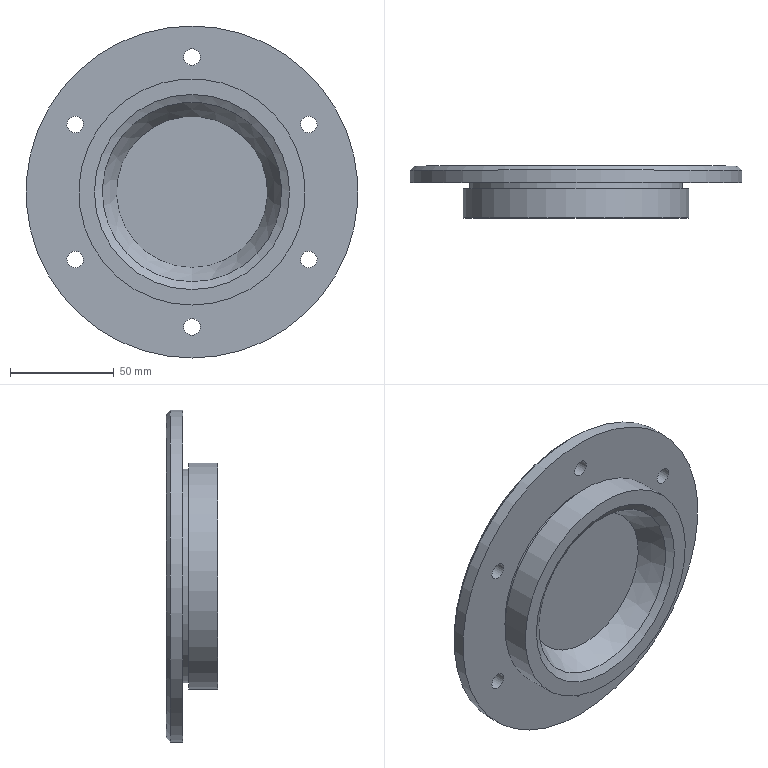Part | NX | features DATUM_CSYS 3, EXTRUDE 3, SKETCH 2, BREP 1 | 1 solid | 19 faces | box 160 x 25 x 160 mm | volume 214093 mm3 | cylinder 9 | plane 6 | cone 4 | commonest cylinder face diameters 8 x6 103 x1 109 x1 160 x1
STEP:
#1=CARTESIAN_POINT('',(0.5,681.,-36.417));
#2=VERTEX_POINT('',#1);
#3=CARTESIAN_POINT('',(0.5,681.,0.));
#4=DIRECTION('',(0.,-1.,0.));
#5=DIRECTION('',(0.,0.,-1.));
#6=AXIS2_PLACEMENT_3D('',#3,#4,#5);
#7=CIRCLE('',#6,36.417);
#8=EDGE_CURVE('',#2,#2,#7,.T.);
#9=ORIENTED_EDGE('',*,*,#8,.F.);
#10=EDGE_LOOP('',(#9));
#11=FACE_BOUND('',#10,.T.);
#12=CARTESIAN_POINT('',(0.5,669.165,-43.25));
#13=VERTEX_POINT('',#12);
#14=CARTESIAN_POINT('',(0.5,669.165,0.));
#15=DIRECTION('',(0.,-1.,0.));
#16=DIRECTION('',(0.,0.,-1.));
#17=AXIS2_PLACEMENT_3D('',#14,#15,#16);
#18=CIRCLE('',#17,43.25);
#19=EDGE_CURVE('',#13,#13,#18,.T.);
#20=ORIENTED_EDGE('',*,*,#19,.T.);
#21=EDGE_LOOP('',(#20));
#22=FACE_BOUND('',#21,.T.);
#23=CARTESIAN_POINT('',(0.5,669.165,0.));
#24=DIRECTION('',(0.,-1.,0.));
#25=DIRECTION('',(0.,0.,-1.));
#26=AXIS2_PLACEMENT_3D('',#23,#24,#25);
#27=CONICAL_SURFACE('',#26,43.25,0.5236);
#28=ADVANCED_FACE('',(#11,#22),#27,.F.);
#29=ORIENTED_EDGE('',*,*,#8,.T.);
#30=EDGE_LOOP('',(#29));
#31=FACE_BOUND('',#30,.T.);
#32=CARTESIAN_POINT('',(36.917,681.,0.));
#33=DIRECTION('',(0.,1.,0.));
#34=DIRECTION('',(0.,0.,1.));
#35=AXIS2_PLACEMENT_3D('',#32,#33,#34);
#36=PLANE('',#35);
#37=ADVANCED_FACE('',(#31),#36,.F.);
#38=CARTESIAN_POINT('',(0.5,689.,-51.));
#39=VERTEX_POINT('',#38);
#40=CARTESIAN_POINT('',(0.5,689.,0.));
#41=DIRECTION('',(0.,-1.,0.));
#42=DIRECTION('',(0.,0.,-1.));
#43=AXIS2_PLACEMENT_3D('',#40,#41,#42);
#44=CIRCLE('',#43,51.);
#45=EDGE_CURVE('',#39,#39,#44,.T.);
#46=ORIENTED_EDGE('',*,*,#45,.F.);
#47=EDGE_LOOP('',(#46));
#48=FACE_BOUND('',#47,.T.);
#49=CARTESIAN_POINT('',(0.5,689.,0.));
#50=DIRECTION('',(0.,-1.,0.));
#51=DIRECTION('',(0.,0.,-1.));
#52=AXIS2_PLACEMENT_3D('',#49,#50,#51);
#53=PLANE('',#52);
#54=ADVANCED_FACE('',(#48),#53,.F.);
#55=CARTESIAN_POINT('',(0.5,692.,-54.));
#56=VERTEX_POINT('',#55);
#57=CARTESIAN_POINT('',(0.5,692.,0.));
#58=DIRECTION('',(0.,-1.,0.));
#59=DIRECTION('',(0.,0.,-1.));
#60=AXIS2_PLACEMENT_3D('',#57,#58,#59);
#61=CIRCLE('',#60,54.);
#62=EDGE_CURVE('',#56,#56,#61,.T.);
#63=ORIENTED_EDGE('',*,*,#62,.F.);
#64=EDGE_LOOP('',(#63));
#65=FACE_BOUND('',#64,.T.);
#66=ORIENTED_EDGE('',*,*,#45,.T.);
#67=EDGE_LOOP('',(#66));
#68=FACE_BOUND('',#67,.T.);
#69=CARTESIAN_POINT('',(0.5,689.,0.));
#70=DIRECTION('',(0.,1.,0.));
#71=DIRECTION('',(0.,0.,1.));
#72=AXIS2_PLACEMENT_3D('',#69,#70,#71);
#73=CONICAL_SURFACE('',#72,51.,0.7854);
#74=ADVANCED_FACE('',(#65,#68),#73,.F.);
#75=CARTESIAN_POINT('',(-57.792,692.,29.036));
#76=VERTEX_POINT('',#75);
#77=CARTESIAN_POINT('',(-55.792,692.,32.5));
#78=DIRECTION('',(0.,1.,0.));
#79=DIRECTION('',(-0.5,0.,-0.866));
#80=AXIS2_PLACEMENT_3D('',#77,#78,#79);
#81=CIRCLE('',#80,4.);
#82=EDGE_CURVE('',#76,#76,#81,.T.);
#83=ORIENTED_EDGE('',*,*,#82,.F.);
#84=EDGE_LOOP('',(#83));
#85=FACE_BOUND('',#84,.T.);
#86=CARTESIAN_POINT('',(4.5,692.,-65.));
#87=VERTEX_POINT('',#86);
#88=CARTESIAN_POINT('',(0.5,692.,-65.));
#89=DIRECTION('',(0.,1.,0.));
#90=DIRECTION('',(1.,0.,0.));
#91=AXIS2_PLACEMENT_3D('',#88,#89,#90);
#92=CIRCLE('',#91,4.);
#93=EDGE_CURVE('',#87,#87,#92,.T.);
#94=ORIENTED_EDGE('',*,*,#93,.F.);
#95=EDGE_LOOP('',(#94));
#96=FACE_BOUND('',#95,.T.);
#97=CARTESIAN_POINT('',(-3.5,692.,65.));
#98=VERTEX_POINT('',#97);
#99=CARTESIAN_POINT('',(0.5,692.,65.));
#100=DIRECTION('',(0.,1.,0.));
#101=DIRECTION('',(-1.,0.,0.));
#102=AXIS2_PLACEMENT_3D('',#99,#100,#101);
#103=CIRCLE('',#102,4.);
#104=EDGE_CURVE('',#98,#98,#103,.T.);
#105=ORIENTED_EDGE('',*,*,#104,.F.);
#106=EDGE_LOOP('',(#105));
#107=FACE_BOUND('',#106,.T.);
#108=CARTESIAN_POINT('',(58.792,692.,-29.036));
#109=VERTEX_POINT('',#108);
#110=CARTESIAN_POINT('',(56.792,692.,-32.5));
#111=DIRECTION('',(0.,1.,0.));
#112=DIRECTION('',(0.5,0.,0.866));
#113=AXIS2_PLACEMENT_3D('',#110,#111,#112);
#114=CIRCLE('',#113,4.);
#115=EDGE_CURVE('',#109,#109,#114,.T.);
#116=ORIENTED_EDGE('',*,*,#115,.F.);
#117=EDGE_LOOP('',(#116));
#118=FACE_BOUND('',#117,.T.);
#119=CARTESIAN_POINT('',(-53.792,692.,-35.964));
#120=VERTEX_POINT('',#119);
#121=CARTESIAN_POINT('',(-55.792,692.,-32.5));
#122=DIRECTION('',(0.,1.,0.));
#123=DIRECTION('',(0.5,0.,-0.866));
#124=AXIS2_PLACEMENT_3D('',#121,#122,#123);
#125=CIRCLE('',#124,4.);
#126=EDGE_CURVE('',#120,#120,#125,.T.);
#127=ORIENTED_EDGE('',*,*,#126,.F.);
#128=EDGE_LOOP('',(#127));
#129=FACE_BOUND('',#128,.T.);
#130=CARTESIAN_POINT('',(54.792,692.,35.964));
#131=VERTEX_POINT('',#130);
#132=CARTESIAN_POINT('',(56.792,692.,32.5));
#133=DIRECTION('',(0.,1.,0.));
#134=DIRECTION('',(-0.5,0.,0.866));
#135=AXIS2_PLACEMENT_3D('',#132,#133,#134);
#136=CIRCLE('',#135,4.);
#137=EDGE_CURVE('',#131,#131,#136,.T.);
#138=ORIENTED_EDGE('',*,*,#137,.F.);
#139=EDGE_LOOP('',(#138));
#140=FACE_BOUND('',#139,.T.);
#141=CARTESIAN_POINT('',(0.5,692.,-78.));
#142=VERTEX_POINT('',#141);
#143=CARTESIAN_POINT('',(0.5,692.,0.));
#144=DIRECTION('',(0.,-1.,0.));
#145=DIRECTION('',(0.,0.,-1.));
#146=AXIS2_PLACEMENT_3D('',#143,#144,#145);
#147=CIRCLE('',#146,78.);
#148=EDGE_CURVE('',#142,#142,#147,.T.);
#149=ORIENTED_EDGE('',*,*,#148,.F.);
#150=EDGE_LOOP('',(#149));
#151=FACE_BOUND('',#150,.T.);
#152=ORIENTED_EDGE('',*,*,#62,.T.);
#153=EDGE_LOOP('',(#152));
#154=FACE_BOUND('',#153,.T.);
#155=CARTESIAN_POINT('',(54.5,692.,0.));
#156=DIRECTION('',(0.,-1.,0.));
#157=DIRECTION('',(0.,0.,-1.));
#158=AXIS2_PLACEMENT_3D('',#155,#156,#157);
#159=PLANE('',#158);
#160=ADVANCED_FACE('',(#85,#96,#107,#118,#129,#140,#151,#154),#159,.F.);
#161=CARTESIAN_POINT('',(0.5,690.,-80.));
#162=VERTEX_POINT('',#161);
#163=CARTESIAN_POINT('',(0.5,690.,0.));
#164=DIRECTION('',(0.,-1.,0.));
#165=DIRECTION('',(0.,0.,-1.));
#166=AXIS2_PLACEMENT_3D('',#163,#164,#165);
#167=CIRCLE('',#166,80.);
#168=EDGE_CURVE('',#162,#162,#167,.T.);
#169=ORIENTED_EDGE('',*,*,#168,.F.);
#170=EDGE_LOOP('',(#169));
#171=FACE_BOUND('',#170,.T.);
#172=ORIENTED_EDGE('',*,*,#148,.T.);
#173=EDGE_LOOP('',(#172));
#174=FACE_BOUND('',#173,.T.);
#175=CARTESIAN_POINT('',(0.5,692.,0.));
#176=DIRECTION('',(0.,-1.,0.));
#177=DIRECTION('',(0.,0.,-1.));
#178=AXIS2_PLACEMENT_3D('',#175,#176,#177);
#179=CONICAL_SURFACE('',#178,78.,0.7854);
#180=ADVANCED_FACE('',(#171,#174),#179,.T.);
#181=CARTESIAN_POINT('',(0.5,684.,-80.));
#182=VERTEX_POINT('',#181);
#183=CARTESIAN_POINT('',(0.5,684.,0.));
#184=DIRECTION('',(0.,-1.,0.));
#185=DIRECTION('',(0.,0.,-1.));
#186=AXIS2_PLACEMENT_3D('',#183,#184,#185);
#187=CIRCLE('',#186,80.);
#188=EDGE_CURVE('',#182,#182,#187,.T.);
#189=ORIENTED_EDGE('',*,*,#188,.F.);
#190=EDGE_LOOP('',(#189));
#191=FACE_BOUND('',#190,.T.);
#192=ORIENTED_EDGE('',*,*,#168,.T.);
#193=EDGE_LOOP('',(#192));
#194=FACE_BOUND('',#193,.T.);
#195=CARTESIAN_POINT('',(0.5,681.,0.));
#196=DIRECTION('',(0.,-1.,0.));
#197=DIRECTION('',(0.,0.,-1.));
#198=AXIS2_PLACEMENT_3D('',#195,#196,#197);
#199=CYLINDRICAL_SURFACE('',#198,80.);
#200=ADVANCED_FACE('',(#191,#194),#199,.T.);
#201=CARTESIAN_POINT('',(-57.792,684.,29.036));
#202=VERTEX_POINT('',#201);
#203=CARTESIAN_POINT('',(-55.792,684.,32.5));
#204=DIRECTION('',(0.,1.,0.));
#205=DIRECTION('',(-0.5,0.,-0.866));
#206=AXIS2_PLACEMENT_3D('',#203,#204,#205);
#207=CIRCLE('',#206,4.);
#208=EDGE_CURVE('',#202,#202,#207,.T.);
#209=ORIENTED_EDGE('',*,*,#208,.T.);
#210=EDGE_LOOP('',(#209));
#211=FACE_BOUND('',#210,.T.);
#212=CARTESIAN_POINT('',(4.5,684.,-65.));
#213=VERTEX_POINT('',#212);
#214=CARTESIAN_POINT('',(0.5,684.,-65.));
#215=DIRECTION('',(0.,1.,0.));
#216=DIRECTION('',(1.,0.,0.));
#217=AXIS2_PLACEMENT_3D('',#214,#215,#216);
#218=CIRCLE('',#217,4.);
#219=EDGE_CURVE('',#213,#213,#218,.T.);
#220=ORIENTED_EDGE('',*,*,#219,.T.);
#221=EDGE_LOOP('',(#220));
#222=FACE_BOUND('',#221,.T.);
#223=CARTESIAN_POINT('',(-3.5,684.,65.));
#224=VERTEX_POINT('',#223);
#225=CARTESIAN_POINT('',(0.5,684.,65.));
#226=DIRECTION('',(0.,1.,0.));
#227=DIRECTION('',(-1.,0.,0.));
#228=AXIS2_PLACEMENT_3D('',#225,#226,#227);
#229=CIRCLE('',#228,4.);
#230=EDGE_CURVE('',#224,#224,#229,.T.);
#231=ORIENTED_EDGE('',*,*,#230,.T.);
#232=EDGE_LOOP('',(#231));
#233=FACE_BOUND('',#232,.T.);
#234=CARTESIAN_POINT('',(58.792,684.,-29.036));
#235=VERTEX_POINT('',#234);
#236=CARTESIAN_POINT('',(56.792,684.,-32.5));
#237=DIRECTION('',(0.,1.,0.));
#238=DIRECTION('',(0.5,0.,0.866));
#239=AXIS2_PLACEMENT_3D('',#236,#237,#238);
#240=CIRCLE('',#239,4.);
#241=EDGE_CURVE('',#235,#235,#240,.T.);
#242=ORIENTED_EDGE('',*,*,#241,.T.);
#243=EDGE_LOOP('',(#242));
#244=FACE_BOUND('',#243,.T.);
#245=CARTESIAN_POINT('',(-53.792,684.,-35.964));
#246=VERTEX_POINT('',#245);
#247=CARTESIAN_POINT('',(-55.792,684.,-32.5));
#248=DIRECTION('',(0.,1.,0.));
#249=DIRECTION('',(0.5,0.,-0.866));
#250=AXIS2_PLACEMENT_3D('',#247,#248,#249);
#251=CIRCLE('',#250,4.);
#252=EDGE_CURVE('',#246,#246,#251,.T.);
#253=ORIENTED_EDGE('',*,*,#252,.T.);
#254=EDGE_LOOP('',(#253));
#255=FACE_BOUND('',#254,.T.);
#256=CARTESIAN_POINT('',(54.792,684.,35.964));
#257=VERTEX_POINT('',#256);
#258=CARTESIAN_POINT('',(56.792,684.,32.5));
#259=DIRECTION('',(0.,1.,0.));
#260=DIRECTION('',(-0.5,0.,0.866));
#261=AXIS2_PLACEMENT_3D('',#258,#259,#260);
#262=CIRCLE('',#261,4.);
#263=EDGE_CURVE('',#257,#257,#262,.T.);
#264=ORIENTED_EDGE('',*,*,#263,.T.);
#265=EDGE_LOOP('',(#264));
#266=FACE_BOUND('',#265,.T.);
#267=CARTESIAN_POINT('',(0.5,684.,-51.5));
#268=VERTEX_POINT('',#267);
#269=CARTESIAN_POINT('',(0.5,684.,0.));
#270=DIRECTION('',(0.,-1.,0.));
#271=DIRECTION('',(0.,0.,-1.));
#272=AXIS2_PLACEMENT_3D('',#269,#270,#271);
#273=CIRCLE('',#272,51.5);
#274=EDGE_CURVE('',#268,#268,#273,.T.);
#275=ORIENTED_EDGE('',*,*,#274,.F.);
#276=EDGE_LOOP('',(#275));
#277=FACE_BOUND('',#276,.T.);
#278=ORIENTED_EDGE('',*,*,#188,.T.);
#279=EDGE_LOOP('',(#278));
#280=FACE_BOUND('',#279,.T.);
#281=CARTESIAN_POINT('',(80.5,684.,0.));
#282=DIRECTION('',(0.,1.,0.));
#283=DIRECTION('',(0.,0.,1.));
#284=AXIS2_PLACEMENT_3D('',#281,#282,#283);
#285=PLANE('',#284);
#286=ADVANCED_FACE('',(#211,#222,#233,#244,#255,#266,#277,#280),#285,.F.);
#287=CARTESIAN_POINT('',(0.5,681.,-51.5));
#288=VERTEX_POINT('',#287);
#289=CARTESIAN_POINT('',(0.5,681.,0.));
#290=DIRECTION('',(0.,-1.,0.));
#291=DIRECTION('',(0.,0.,-1.));
#292=AXIS2_PLACEMENT_3D('',#289,#290,#291);
#293=CIRCLE('',#292,51.5);
#294=EDGE_CURVE('',#288,#288,#293,.T.);
#295=ORIENTED_EDGE('',*,*,#294,.F.);
#296=EDGE_LOOP('',(#295));
#297=FACE_BOUND('',#296,.T.);
#298=ORIENTED_EDGE('',*,*,#274,.T.);
#299=EDGE_LOOP('',(#298));
#300=FACE_BOUND('',#299,.T.);
#301=CARTESIAN_POINT('',(0.5,681.,0.));
#302=DIRECTION('',(0.,-1.,0.));
#303=DIRECTION('',(0.,0.,-1.));
#304=AXIS2_PLACEMENT_3D('',#301,#302,#303);
#305=CYLINDRICAL_SURFACE('',#304,51.5);
#306=ADVANCED_FACE('',(#297,#300),#305,.T.);
#307=CARTESIAN_POINT('',(0.5,681.,-54.5));
#308=VERTEX_POINT('',#307);
#309=CARTESIAN_POINT('',(0.5,681.,0.));
#310=DIRECTION('',(0.,-1.,0.));
#311=DIRECTION('',(0.,0.,-1.));
#312=AXIS2_PLACEMENT_3D('',#309,#310,#311);
#313=CIRCLE('',#312,54.5);
#314=EDGE_CURVE('',#308,#308,#313,.T.);
#315=ORIENTED_EDGE('',*,*,#314,.F.);
#316=EDGE_LOOP('',(#315));
#317=FACE_BOUND('',#316,.T.);
#318=ORIENTED_EDGE('',*,*,#294,.T.);
#319=EDGE_LOOP('',(#318));
#320=FACE_BOUND('',#319,.T.);
#321=CARTESIAN_POINT('',(52.,681.,0.));
#322=DIRECTION('',(0.,-1.,0.));
#323=DIRECTION('',(0.,0.,-1.));
#324=AXIS2_PLACEMENT_3D('',#321,#322,#323);
#325=PLANE('',#324);
#326=ADVANCED_FACE('',(#317,#320),#325,.F.);
#327=CARTESIAN_POINT('',(0.5,667.,-54.5));
#328=VERTEX_POINT('',#327);
#329=CARTESIAN_POINT('',(0.5,667.,0.));
#330=DIRECTION('',(0.,-1.,0.));
#331=DIRECTION('',(0.,0.,-1.));
#332=AXIS2_PLACEMENT_3D('',#329,#330,#331);
#333=CIRCLE('',#332,54.5);
#334=EDGE_CURVE('',#328,#328,#333,.T.);
#335=ORIENTED_EDGE('',*,*,#334,.F.);
#336=EDGE_LOOP('',(#335));
#337=FACE_BOUND('',#336,.T.);
#338=ORIENTED_EDGE('',*,*,#314,.T.);
#339=EDGE_LOOP('',(#338));
#340=FACE_BOUND('',#339,.T.);
#341=CARTESIAN_POINT('',(0.5,681.,0.));
#342=DIRECTION('',(0.,-1.,0.));
#343=DIRECTION('',(0.,0.,-1.));
#344=AXIS2_PLACEMENT_3D('',#341,#342,#343);
#345=CYLINDRICAL_SURFACE('',#344,54.5);
#346=ADVANCED_FACE('',(#337,#340),#345,.T.);
#347=CARTESIAN_POINT('',(0.5,667.,-47.));
#348=VERTEX_POINT('',#347);
#349=CARTESIAN_POINT('',(0.5,667.,0.));
#350=DIRECTION('',(0.,-1.,0.));
#351=DIRECTION('',(0.,0.,-1.));
#352=AXIS2_PLACEMENT_3D('',#349,#350,#351);
#353=CIRCLE('',#352,47.);
#354=EDGE_CURVE('',#348,#348,#353,.T.);
#355=ORIENTED_EDGE('',*,*,#354,.F.);
#356=EDGE_LOOP('',(#355));
#357=FACE_BOUND('',#356,.T.);
#358=ORIENTED_EDGE('',*,*,#334,.T.);
#359=EDGE_LOOP('',(#358));
#360=FACE_BOUND('',#359,.T.);
#361=CARTESIAN_POINT('',(55.,667.,0.));
#362=DIRECTION('',(0.,1.,0.));
#363=DIRECTION('',(0.,0.,1.));
#364=AXIS2_PLACEMENT_3D('',#361,#362,#363);
#365=PLANE('',#364);
#366=ADVANCED_FACE('',(#357,#360),#365,.F.);
#367=ORIENTED_EDGE('',*,*,#19,.F.);
#368=EDGE_LOOP('',(#367));
#369=FACE_BOUND('',#368,.T.);
#370=ORIENTED_EDGE('',*,*,#354,.T.);
#371=EDGE_LOOP('',(#370));
#372=FACE_BOUND('',#371,.T.);
#373=CARTESIAN_POINT('',(0.5,667.,0.));
#374=DIRECTION('',(0.,-1.,0.));
#375=DIRECTION('',(0.,0.,-1.));
#376=AXIS2_PLACEMENT_3D('',#373,#374,#375);
#377=CONICAL_SURFACE('',#376,47.,1.047);
#378=ADVANCED_FACE('',(#369,#372),#377,.F.);
#379=ORIENTED_EDGE('',*,*,#263,.F.);
#380=EDGE_LOOP('',(#379));
#381=FACE_BOUND('',#380,.T.);
#382=ORIENTED_EDGE('',*,*,#137,.T.);
#383=EDGE_LOOP('',(#382));
#384=FACE_BOUND('',#383,.T.);
#385=CARTESIAN_POINT('',(56.792,684.,32.5));
#386=DIRECTION('',(0.,1.,0.));
#387=DIRECTION('',(0.,0.,1.));
#388=AXIS2_PLACEMENT_3D('',#385,#386,#387);
#389=CYLINDRICAL_SURFACE('',#388,4.);
#390=ADVANCED_FACE('',(#381,#384),#389,.F.);
#391=ORIENTED_EDGE('',*,*,#252,.F.);
#392=EDGE_LOOP('',(#391));
#393=FACE_BOUND('',#392,.T.);
#394=ORIENTED_EDGE('',*,*,#126,.T.);
#395=EDGE_LOOP('',(#394));
#396=FACE_BOUND('',#395,.T.);
#397=CARTESIAN_POINT('',(-55.792,684.,-32.5));
#398=DIRECTION('',(0.,1.,0.));
#399=DIRECTION('',(0.,0.,1.));
#400=AXIS2_PLACEMENT_3D('',#397,#398,#399);
#401=CYLINDRICAL_SURFACE('',#400,4.);
#402=ADVANCED_FACE('',(#393,#396),#401,.F.);
#403=ORIENTED_EDGE('',*,*,#241,.F.);
#404=EDGE_LOOP('',(#403));
#405=FACE_BOUND('',#404,.T.);
#406=ORIENTED_EDGE('',*,*,#115,.T.);
#407=EDGE_LOOP('',(#406));
#408=FACE_BOUND('',#407,.T.);
#409=CARTESIAN_POINT('',(56.792,684.,-32.5));
#410=DIRECTION('',(0.,1.,0.));
#411=DIRECTION('',(0.,0.,1.));
#412=AXIS2_PLACEMENT_3D('',#409,#410,#411);
#413=CYLINDRICAL_SURFACE('',#412,4.);
#414=ADVANCED_FACE('',(#405,#408),#413,.F.);
#415=ORIENTED_EDGE('',*,*,#230,.F.);
#416=EDGE_LOOP('',(#415));
#417=FACE_BOUND('',#416,.T.);
#418=ORIENTED_EDGE('',*,*,#104,.T.);
#419=EDGE_LOOP('',(#418));
#420=FACE_BOUND('',#419,.T.);
#421=CARTESIAN_POINT('',(0.5,684.,65.));
#422=DIRECTION('',(0.,1.,0.));
#423=DIRECTION('',(0.,0.,1.));
#424=AXIS2_PLACEMENT_3D('',#421,#422,#423);
#425=CYLINDRICAL_SURFACE('',#424,4.);
#426=ADVANCED_FACE('',(#417,#420),#425,.F.);
#427=ORIENTED_EDGE('',*,*,#219,.F.);
#428=EDGE_LOOP('',(#427));
#429=FACE_BOUND('',#428,.T.);
#430=ORIENTED_EDGE('',*,*,#93,.T.);
#431=EDGE_LOOP('',(#430));
#432=FACE_BOUND('',#431,.T.);
#433=CARTESIAN_POINT('',(0.5,684.,-65.));
#434=DIRECTION('',(0.,1.,0.));
#435=DIRECTION('',(0.,0.,1.));
#436=AXIS2_PLACEMENT_3D('',#433,#434,#435);
#437=CYLINDRICAL_SURFACE('',#436,4.);
#438=ADVANCED_FACE('',(#429,#432),#437,.F.);
#439=ORIENTED_EDGE('',*,*,#208,.F.);
#440=EDGE_LOOP('',(#439));
#441=FACE_BOUND('',#440,.T.);
#442=ORIENTED_EDGE('',*,*,#82,.T.);
#443=EDGE_LOOP('',(#442));
#444=FACE_BOUND('',#443,.T.);
#445=CARTESIAN_POINT('',(-55.792,684.,32.5));
#446=DIRECTION('',(0.,1.,0.));
#447=DIRECTION('',(0.,0.,1.));
#448=AXIS2_PLACEMENT_3D('',#445,#446,#447);
#449=CYLINDRICAL_SURFACE('',#448,4.);
#450=ADVANCED_FACE('',(#441,#444),#449,.F.);
#451=CLOSED_SHELL('',(#28,#37,#54,#74,#160,#180,#200,#286,#306,#326,#346,#366,#378,#390,#402,#414,#426,#438,#450));
#452=MANIFOLD_SOLID_BREP('',#451);
#453=(LENGTH_UNIT()NAMED_UNIT(*)SI_UNIT(.MILLI.,.METRE.));
#454=UNCERTAINTY_MEASURE_WITH_UNIT(LENGTH_MEASURE(0.00001),#453,'','');
#455=(NAMED_UNIT(*)PLANE_ANGLE_UNIT()SI_UNIT($,.RADIAN.));
#456=(NAMED_UNIT(*)SI_UNIT($,.STERADIAN.)SOLID_ANGLE_UNIT());
#457=(GEOMETRIC_REPRESENTATION_CONTEXT(3)GLOBAL_UNCERTAINTY_ASSIGNED_CONTEXT((#454))GLOBAL_UNIT_ASSIGNED_CONTEXT((#453,#455,#456))REPRESENTATION_CONTEXT('',''));
#458=ADVANCED_BREP_SHAPE_REPRESENTATION('',(#452),#457);